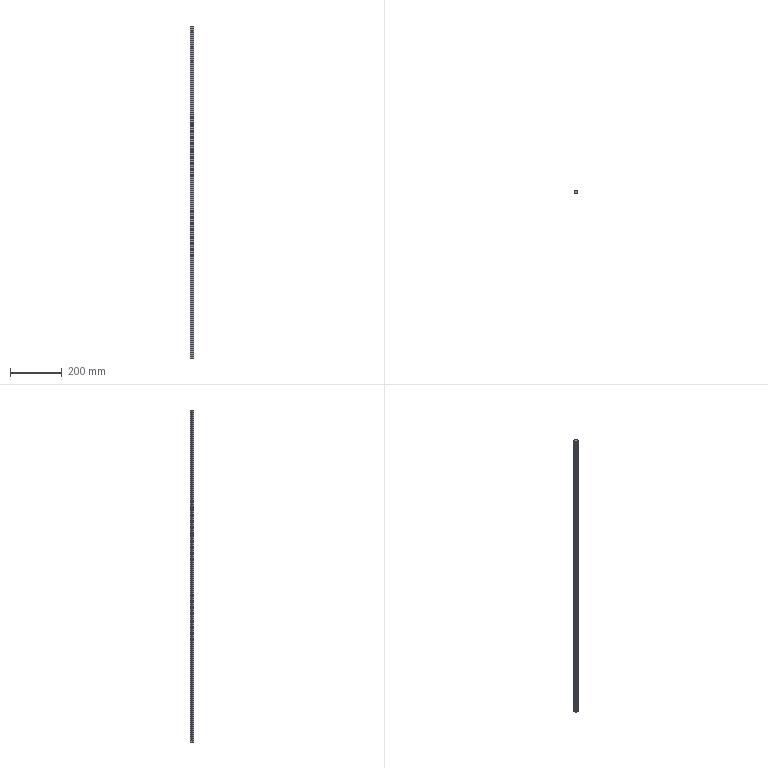Part | STEP file | EG15_RAIL-2 | 1 solid | 53 faces | box 15 x 12.5 x 1282 mm | volume 208724 mm3 | cylinder 30 | plane 23 | commonest cylinder face diameters 0.6 x11 3.5 x6 6 x6 3 x5 1 x2